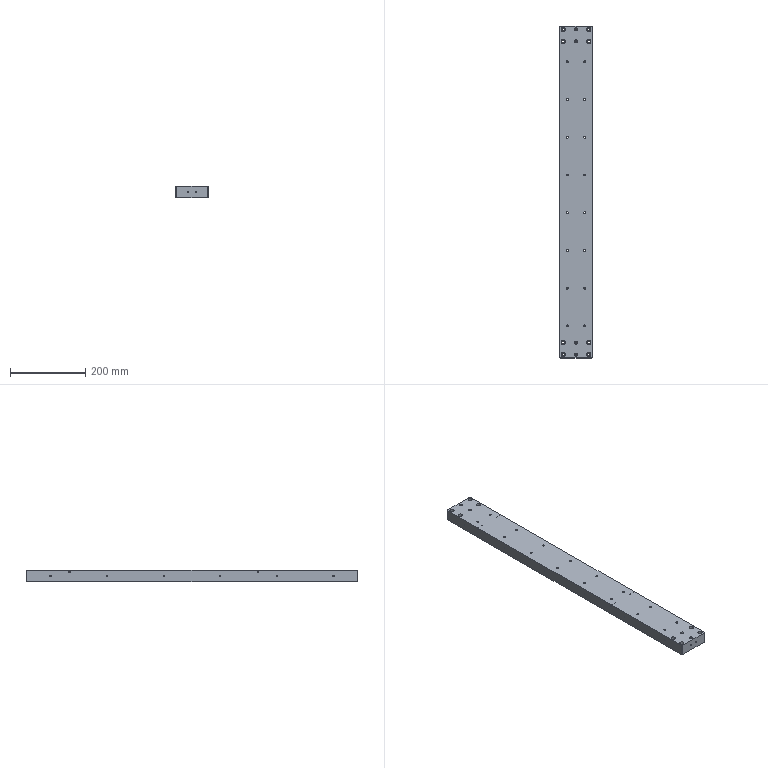Part | STEP file | 1 solid | 174 faces | box 86 x 880 x 30 mm | volume 2237479 mm3 | cylinder 116 | cone 36 | plane 22 | commonest cylinder face diameters 5 x40 3.3 x24 6.6 x16 11 x16 4.2 x8 8 x8